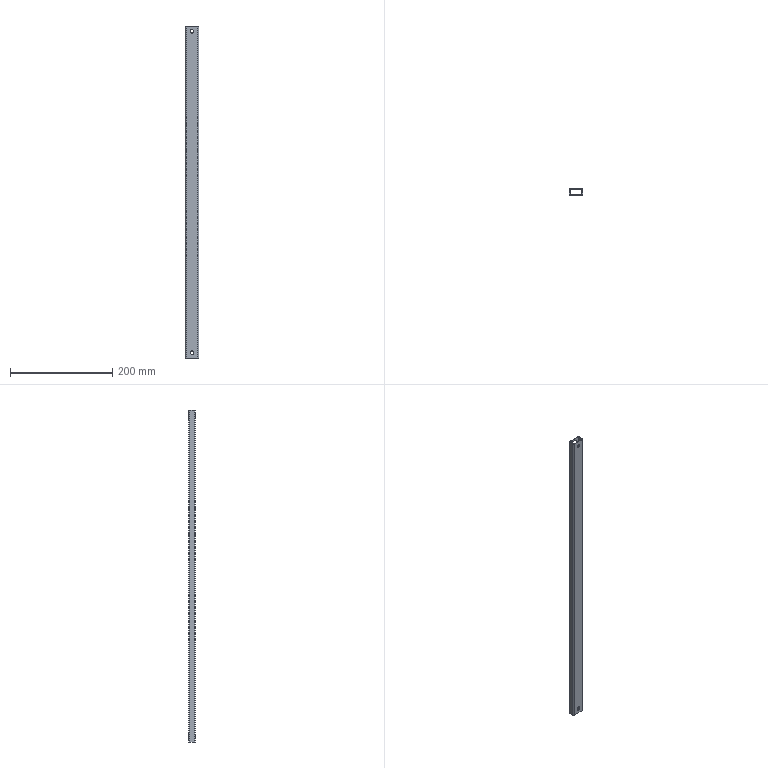Part | STEP file | Q7C0901 | 1 solid | 22 faces | box 26 x 13 x 648 mm | volume 67252 mm3 | cylinder 12 | plane 10 | commonest cylinder face diameters 1 x4 4 x4 7 x2 15 x2